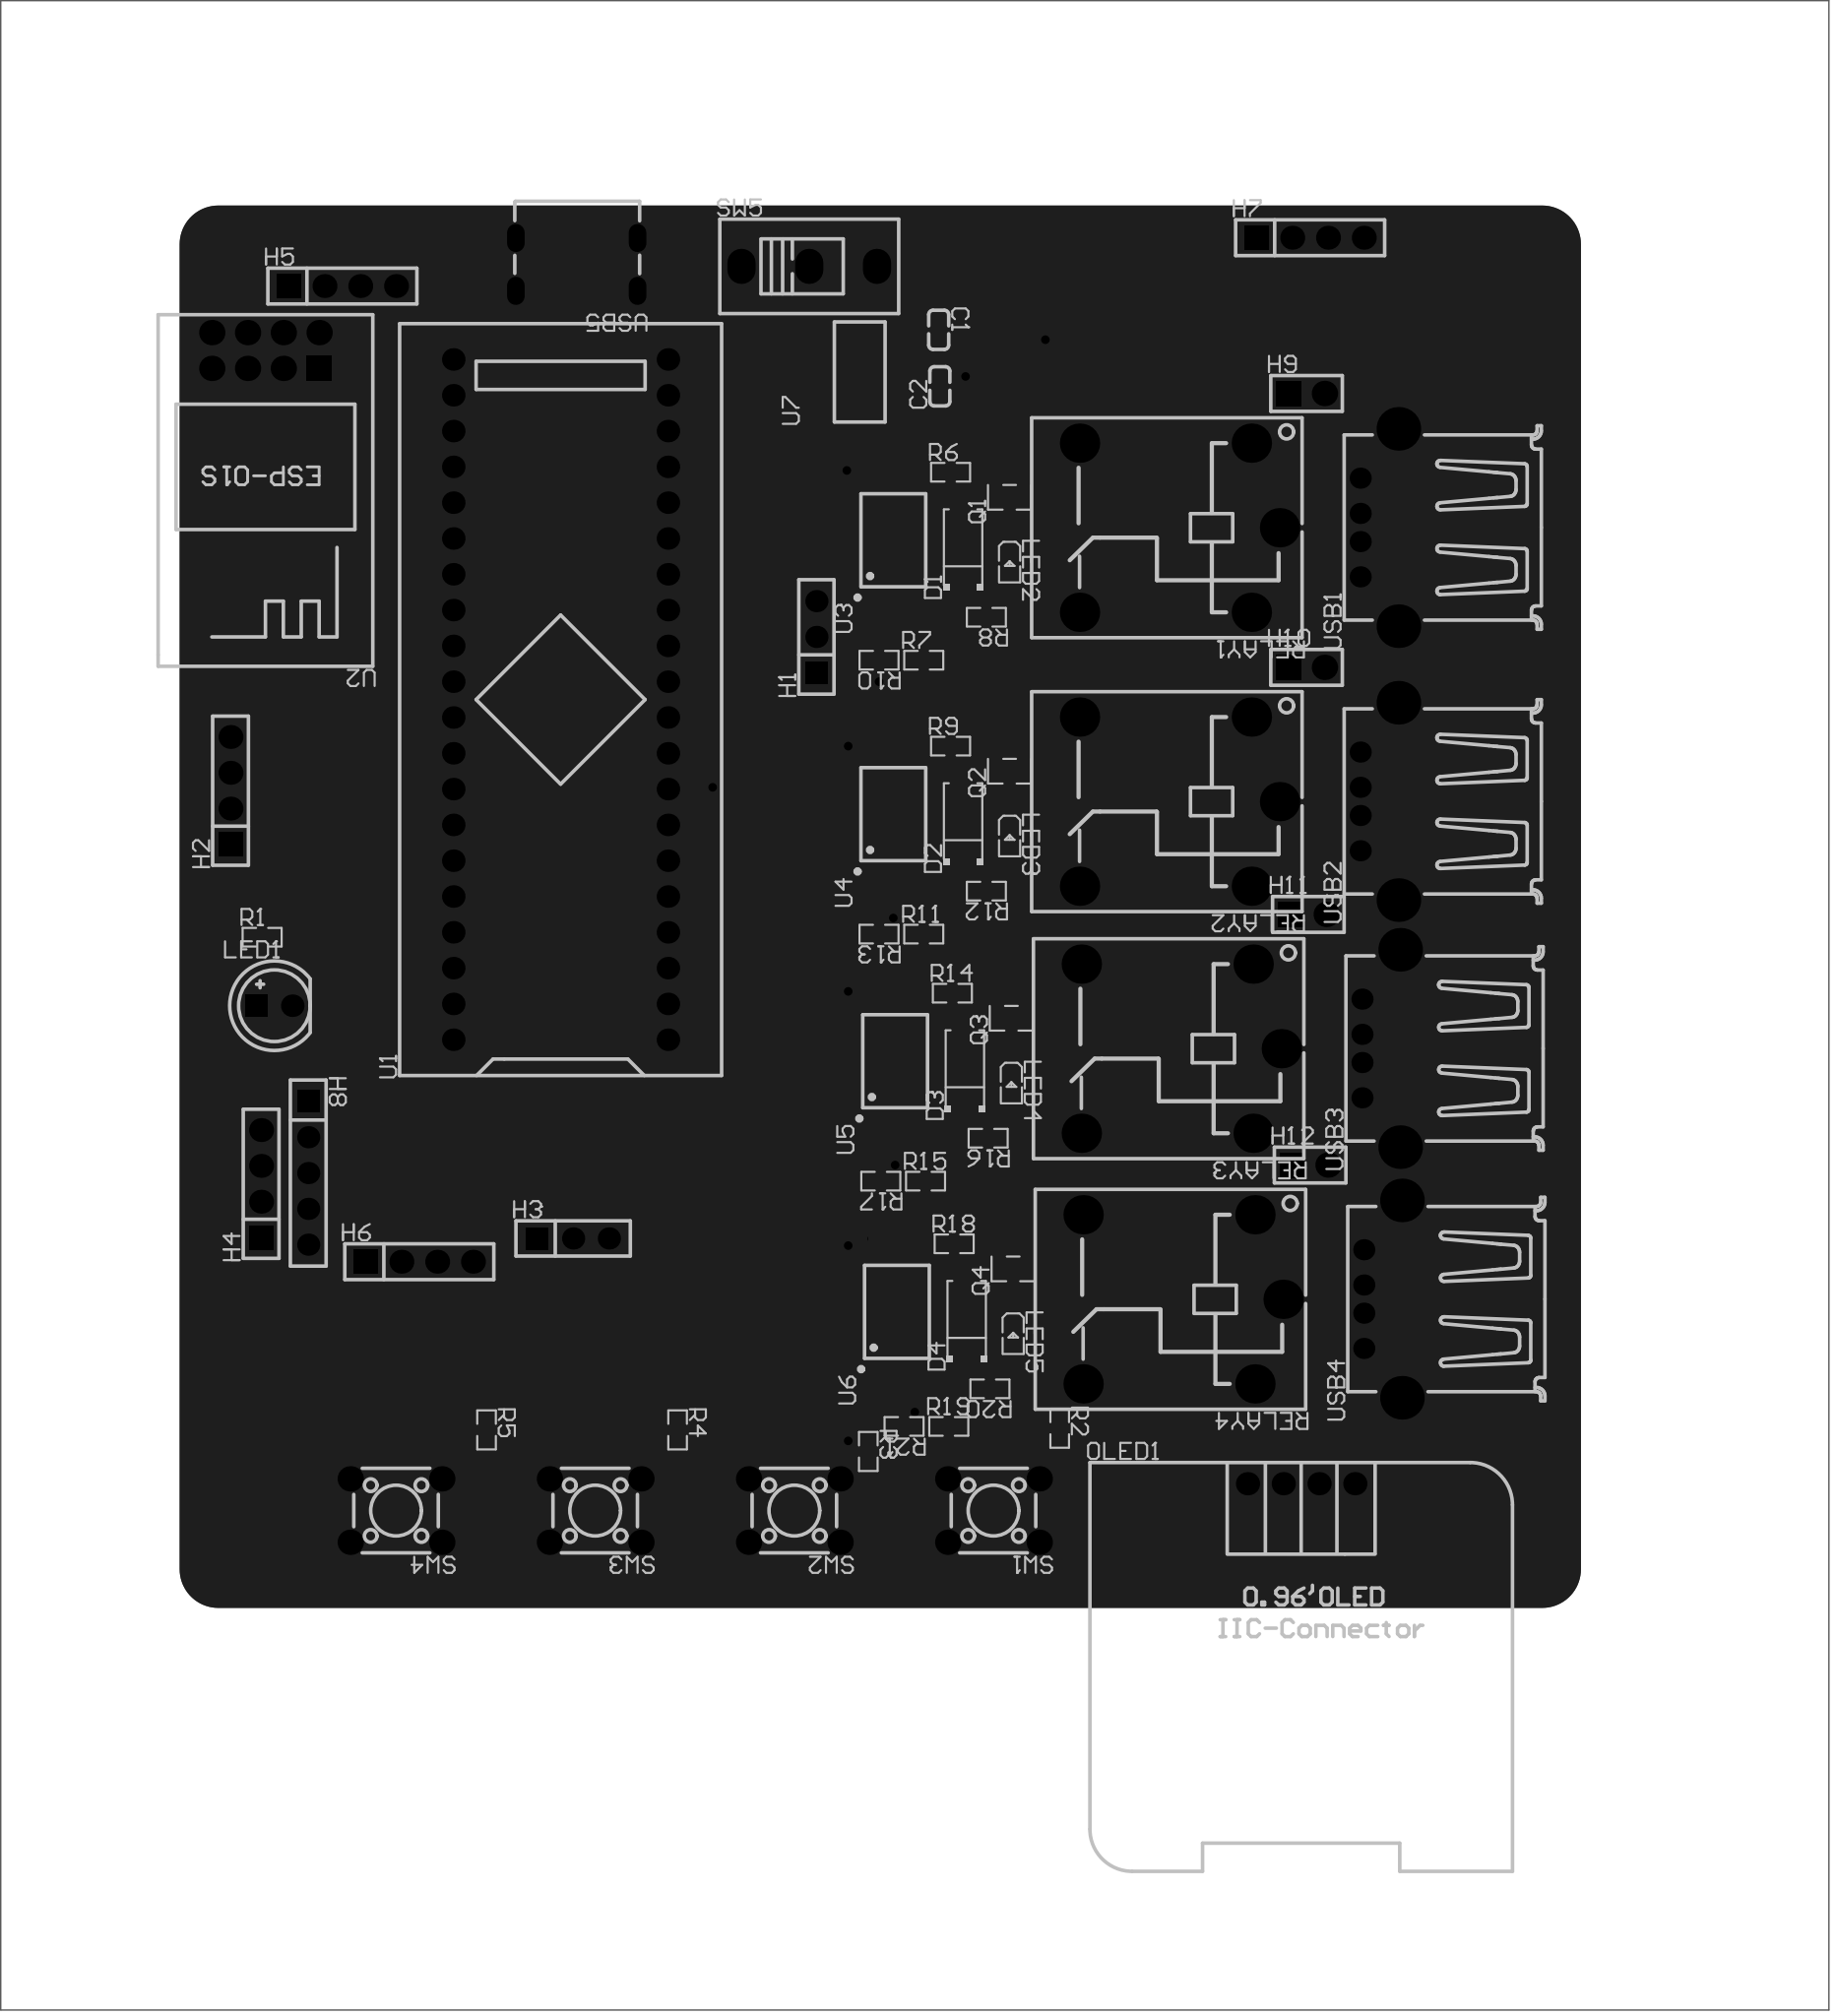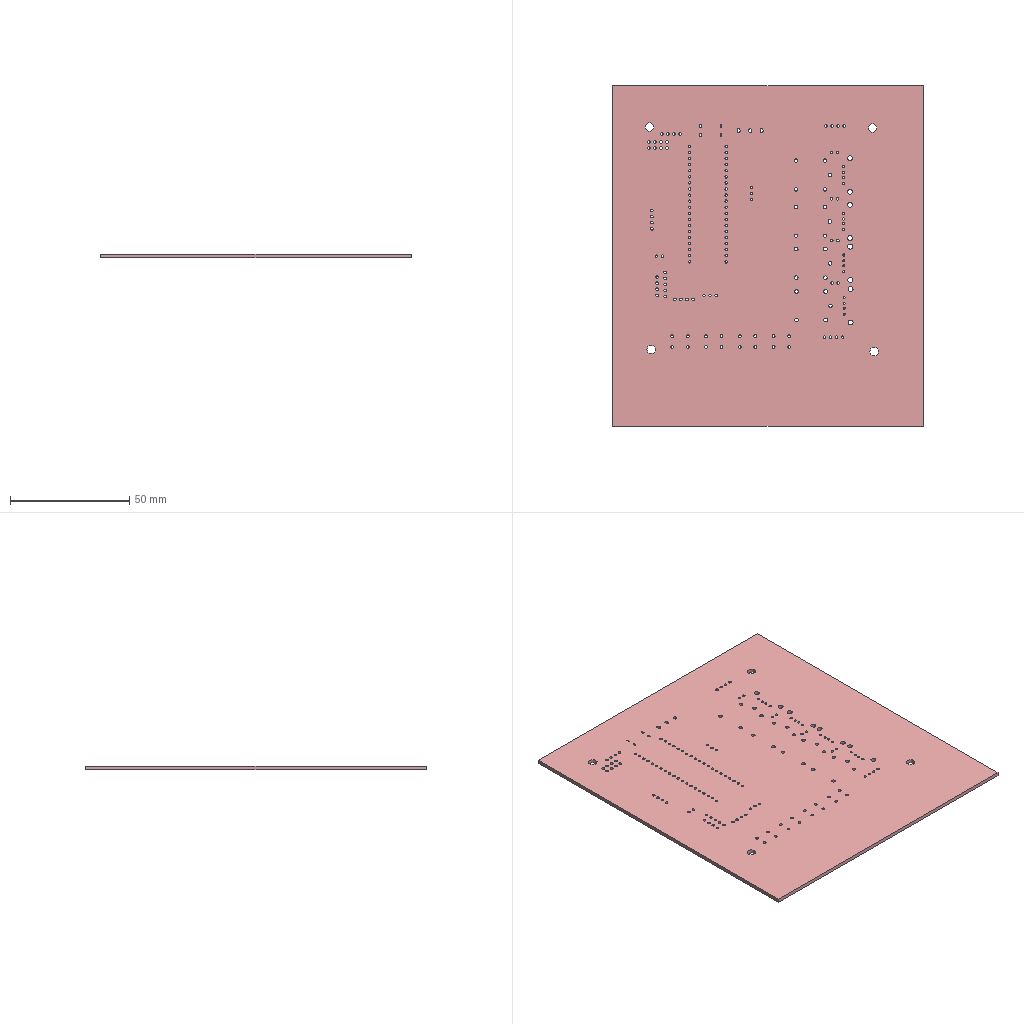Circuit board layout | Altium Designer | box 129.8 x 142.5 x 1.6 mm
Layer stack:
# Altium Designer layer stack of  (unit mm; dielectric type: 0 none, 1 core, 2 prepreg, 3 surface material)
index,name,kind,layer,copper_thickness_mm,dielectric_type,dielectric_thickness_mm,dielectric_material,dielectric_constant
0,Top Paste Mask Layer,other,,,,,,
1,Top Silkscreen Layer,other,,,,,,
2,Top Solder Mask Layer,dielectric,,,3,0.01,,3.3
3,Top Layer,copper,Top Layer,0.035,,,,
4,Dielectric1,dielectric,,,3,1.51,FR4,4.5
5,Bottom Layer,copper,Bottom Layer,0.035,,,,
6,Bottom Solder Mask Layer,dielectric,,,3,0.01,,3.3
7,Bottom Silkscreen Layer,other,,,,,,
8,Bottom Paste Mask Layer,other,,,,,,
# drill layer pairs: low layer,high layer
drill_pair,Top Layer,Bottom Layer
Part placement:
Designator,Comment,Layer,Footprint,Center-X(mm),Center-Y(mm),Rotation
C1,100nF,TopLayer,C0603,136.444,189.046,270
C2,100nF,TopLayer,C0603,136.525,185.039,90
D1,US1M,TopLayer,SMA_L4.4-W2.8-LS5.4-RD,138.176,173.609,90
D2,US1M,TopLayer,SMA_L4.4-W2.8-LS5.4-RD,138.176,154.178,90
D3,US1M,TopLayer,SMA_L4.4-W2.8-LS5.4-RD,138.303,136.652,90
D4,US1M,TopLayer,SMA_L4.4-W2.8-LS5.4-RD,138.43,118.872,90
H1,,TopLayer,HDR-TH_3P-P2.54-V-F,127.762,167.259,90
H2,,TopLayer,HDR-TH_4P-P2.54-V-F,86.166,156.351,90
H3,,TopLayer,HDR-TH_3P-P2.54-V-F,110.49,124.587,0
H4,,TopLayer,HDR-TH_4P-P2.54-V-F,88.337,128.464,90
H5,,TopLayer,HDR-TH_4P-P2.54-V-F,94.107,192.151,0
H6,,TopLayer,HDR-TH_4P-P2.54-V-F,99.568,122.936,0
H7,,TopLayer,HDR-TH_4P-P2.54-V-F,162.814,195.58,0
H8,,TopLayer,HDR-TH_5P-P2.54-V-F,91.683,129.226,270
H9,,TopLayer,HDR-TH_2P-P2.54-V-M-1,162.56,184.531,0
H10,,TopLayer,HDR-TH_2P-P2.54-V-M-1,162.56,165.1,0
H11,,TopLayer,HDR-TH_2P-P2.54-V-M-1,162.687,147.574,0
H12,,TopLayer,HDR-TH_2P-P2.54-V-M-1,162.814,129.794,0
LED1,,TopLayer,LED-TH_5mm,89.281,141.097,0
OLED1,,TopLayer,0.96OLED_4P,162.179,107.188,0
Q1,S8050,TopLayer,SOT-23-3_L2.9-W1.6-P1.90-LS2.8-BR,141.478,177.165,90
Q2,S8050,TopLayer,SOT-23-3_L2.9-W1.6-P1.90-LS2.8-BR,141.478,157.734,90
Q3,S8050,TopLayer,SOT-23-3_L2.9-W1.6-P1.90-LS2.8-BR,141.605,140.208,90
Q4,S8050,TopLayer,SOT-23-3_L2.9-W1.6-P1.90-LS2.8-BR,141.732,122.428,90
R1,10K,TopLayer,R0603,88.409,145.956,0
R2,10K,TopLayer,R0603,145.034,111.125,270
R3,10K,TopLayer,R0603,131.445,109.474,270
R4,10K,TopLayer,R0603,117.906,111.005,270
R5,10K,TopLayer,R0603,104.342,111.005,270
R6,1kΩ,TopLayer,R0603,137.287,178.943,0
R7,470Ω,TopLayer,R0603,135.382,165.608,0
R8,4.7kΩ,TopLayer,R0603,139.827,168.656,180
R9,1kΩ,TopLayer,R0603,137.287,159.512,0
R10,1kΩ,TopLayer,R0603,132.207,165.608,180
R11,470Ω,TopLayer,R0603,135.382,146.177,0
R12,4.7kΩ,TopLayer,R0603,139.827,149.225,180
R13,1kΩ,TopLayer,R0603,132.207,146.177,180
R14,1kΩ,TopLayer,R0603,137.414,141.986,0
R15,470Ω,TopLayer,R0603,135.509,128.651,0
R16,4.7kΩ,TopLayer,R0603,139.954,131.699,180
R17,1kΩ,TopLayer,R0603,132.334,128.651,180
R18,1kΩ,TopLayer,R0603,137.541,124.206,0
R19,470Ω,TopLayer,R0603,137.16,111.252,0
R20,4.7kΩ,TopLayer,R0603,140.081,113.919,180
R21,1kΩ,TopLayer,R0603,133.985,111.252,180
RELAY1,SRD-12VDC-SL-C,TopLayer,RELAY-TH_SRD-XXVDC-XL-C,153.543,175.006,180
RELAY2,SRD-12VDC-SL-C,TopLayer,RELAY-TH_SRD-XXVDC-XL-C,153.543,155.575,180
RELAY3,SRD-12VDC-SL-C,TopLayer,RELAY-TH_SRD-XXVDC-XL-C,153.67,138.049,180
RELAY4,SRD-12VDC-SL-C,TopLayer,RELAY-TH_SRD-XXVDC-XL-C,153.797,120.269,180
SW1,,TopLayer,SW-TH_4P-L6.0-W6.0-P4.50-LS6.5,140.335,105.283,180
SW2,,TopLayer,SW-TH_4P-L6.0-W6.0-P4.50-LS6.5,126.196,105.283,180
SW3,,TopLayer,SW-TH_4P-L6.0-W6.0-P4.50-LS6.5,112.056,105.283,180
SW4,,TopLayer,SW-TH_4P-L6.0-W6.0-P4.50-LS6.5,97.917,105.283,180
SW5,XY-SS12D10L3,TopLayer,SW-TH_3P-L12.7-W6.7_XY-SS12D10LXX,127.254,193.548,0
U1,STM32F103C8T6-Card,TopLayer,CONN-TH_L53.3-W22.9_STM32F103C8T6-CARD,109.601,162.814,90
U2,ESP-01S,TopLayer,WIFIM-TH_ESP-01S,88.646,187.579,180
U3,PC817C,TopLayer,OPTO-SMD-4_L4.6-W6.5-P2.54-LS10.3-TL,133.223,174.117,90
U4,PC817C,TopLayer,OPTO-SMD-4_L4.6-W6.5-P2.54-LS10.3-TL,133.223,154.686,90
U5,PC817C,TopLayer,OPTO-SMD-4_L4.6-W6.5-P2.54-LS10.3-TL,133.35,137.16,90
U6,PC817C,TopLayer,OPTO-SMD-4_L4.6-W6.5-P2.54-LS10.3-TL,133.477,119.38,90
U7,,TopLayer,SOT_223,130.837,186.056,90
USB1,,TopLayer,USB__Type-A,167.725,175.022,90
USB2,,TopLayer,USB__Type-A,167.725,155.591,90
USB3,,TopLayer,USB__Type-A,167.852,138.065,90
USB4,,TopLayer,USB__Type-A,167.979,120.285,90
USB5,,TopLayer,USB__TYPE-C-6P,110.744,193.421,180
LED2,,TopLayer,LED_0603,141.47,172.517,270
LED3,,TopLayer,LED_0603,141.47,153.086,270
LED4,,TopLayer,LED_0603,141.597,135.56,270
LED5,,TopLayer,LED_0603,141.724,117.78,270
Pad and via stacks:
# Altium Designer via and pad stacks of  (unit mm). Each distinct definition once, with the count of objects using it.
# via: kind,start_layer,end_layer,hole_mm,diameter_mm,mode(0 simple;1 top-mid-bottom;2 full stack),diameter_per_layer,count,example_net
# pad: kind,layer,hole_mm,hole_type(0 round;1 square;2 slot),plating,top_size,top_shape(1 round;2 rect;3 octagon;9 rounded rect),mid_size,bottom_size,mode,footprint,size_per_layer,count,example
pad,Top Layer,0,0,plated,0.8x0.9,2,0.8x0.9,0.8x0.9,0,C0603,,4,C1.2
pad,Top Layer,0,0,plated,2.046x1.62,2,2.046x1.62,2.046x1.62,0,SMA_L4.4-W2.8-LS5.4-RD,,8,D1.2
pad,Top Layer,0,0,plated,1.07x0.6,2,1.07x0.6,1.07x0.6,0,SOT-23-3_L2.9-W1.6-P1.90-LS2.8-BR,,12,Q1.1
pad,Top Layer,0,0,plated,0.8065x0.864,2,0.8065x0.864,0.8065x0.864,0,R0603,,42,R1.2
pad,Top Layer,0,0,plated,1.5x3,2,1.5x3,1.5x3,0,OPTO-SMD-4_L4.6-W6.5-P2.54-LS10.3-TL,,16,U3.4
pad,Top Layer,0,0,plated,2.2x3.5,2,2.2x3.5,2.2x3.5,0,SOT_223,,1,U7.4
pad,Top Layer,0,0,plated,1.1x2.2,2,1.1x2.2,1.1x2.2,0,SOT_223,,3,U7.3
pad,Top Layer,0,0,plated,0.7x1.2,2,0.7x1.2,0.7x1.2,0,USB_ TYPE-C-6P,,2,USB5.A5
pad,Top Layer,0,0,plated,0.8x1.2,2,0.8x1.2,0.8x1.2,0,USB_ TYPE-C-6P,,2,USB5.B9
pad,Top Layer,0,0,plated,0.9x1.2,2,0.9x1.2,0.9x1.2,0,USB_ TYPE-C-6P,,2,USB5.B12
pad,Top Layer,0,0,plated,0.8001x0.8001,2,0.8001x0.8001,0.8001x0.8001,0,LED_0603,,8,LED2.1
pad,Multi-Layer,1.02,0,plated,1.575x1.575,1,1.575x1.575,1.575x1.575,0,HDR-TH_3P-P2.54-V-F,,4,H1.3
pad,Multi-Layer,1.02,0,plated,1.575x1.575,2,1.575x1.575,1.575x1.575,0,HDR-TH_3P-P2.54-V-F,,2,H1.1
pad,Multi-Layer,1.1,0,plated,1.7x1.7,2,1.7x1.7,1.7x1.7,0,HDR-TH_4P-P2.54-V-F,,5,H2.1
pad,Multi-Layer,1.1,0,plated,1.7x1.7,1,1.7x1.7,1.7x1.7,0,HDR-TH_4P-P2.54-V-F,,15,H2.2
pad,Multi-Layer,1.02,0,plated,1.575x1.575,1,1.575x1.575,1.575x1.575,0,HDR-TH_5P-P2.54-V-F,,4,H8.5
pad,Multi-Layer,1.02,0,plated,1.575x1.575,2,1.575x1.575,1.575x1.575,0,HDR-TH_5P-P2.54-V-F,,1,H8.1
pad,Multi-Layer,1.1,0,plated,1.8x1.8,1,1.8x1.8,1.8x1.8,0,HDR-TH_2P-P2.54-V-M-1,,4,H9.2
pad,Multi-Layer,1.1,0,plated,1.8x1.8,2,1.8x1.8,1.8x1.8,0,HDR-TH_2P-P2.54-V-M-1,,4,H9.1
pad,Multi-Layer,1,0,plated,1.6x1.6,2,1.6x1.6,1.6x1.6,0,LED-TH_5mm,,1,LED1.1
pad,Multi-Layer,1,0,plated,1.6x1.6,1,1.6x1.6,1.6x1.6,0,LED-TH_5mm,,1,LED1.2
pad,Multi-Layer,1,0,plated,1.65x1.65,1,1.65x1.65,1.65x1.65,0,0.96OLED_4P,,4,OLED1.4
pad,Multi-Layer,1.524,0,plated,2.794x2.794,1,2.794x2.794,2.794x2.794,0,RELAY-TH_SRD-XXVDC-XL-C,,20,RELAY1.2
pad,Multi-Layer,1.2,0,plated,1.8x1.8,1,1.8x1.8,1.8x1.8,0,SW-TH_4P-L6.0-W6.0-P4.50-LS6.5,,16,SW1.1
pad,Multi-Layer,1.2,2,plated,2x2.5,1,2x2.5,2x2.5,0,SW-TH_3P-L12.7-W6.7_XY-SS12D10LXX,,3,SW5.1
pad,Multi-Layer,1,0,plated,1.6x1.6,1,1.6x1.6,1.6x1.6,0,CONN-TH_L53.3-W22.9_STM32F103C8T6-CARD,,40,U1.1
pad,Multi-Layer,1.2,0,plated,1.8x1.8,2,1.8x1.8,1.8x1.8,0,WIFIM-TH_ESP-01S,,1,U2.1
pad,Multi-Layer,1.2,0,plated,1.8x1.8,1,1.8x1.8,1.8x1.8,0,WIFIM-TH_ESP-01S,,7,U2.2
pad,Multi-Layer,2.1,0,plated,3.1x3.1,1,3.1x3.1,3.1x3.1,0,USB_ Type-A,,8,USB1.SH2
pad,Multi-Layer,0.9,0,plated,1.5x1.5,1,1.5x1.5,1.5x1.5,0,USB_ Type-A,,16,USB1.1
pad,Multi-Layer,0.6,2,plated,1.25x2,1,1.25x2,1.25x2,0,USB_ TYPE-C-6P,,4,USB5.8
via,Top Layer,Bottom Layer,0.3048,0.61,0,,13,PA11
Copper pours:
name,layer,net,type(0 solid;1 hatched;2 none)
Top Layer-GND,Top Layer,GND,0
Bottom Layer-GND,Bottom Layer,GND,0